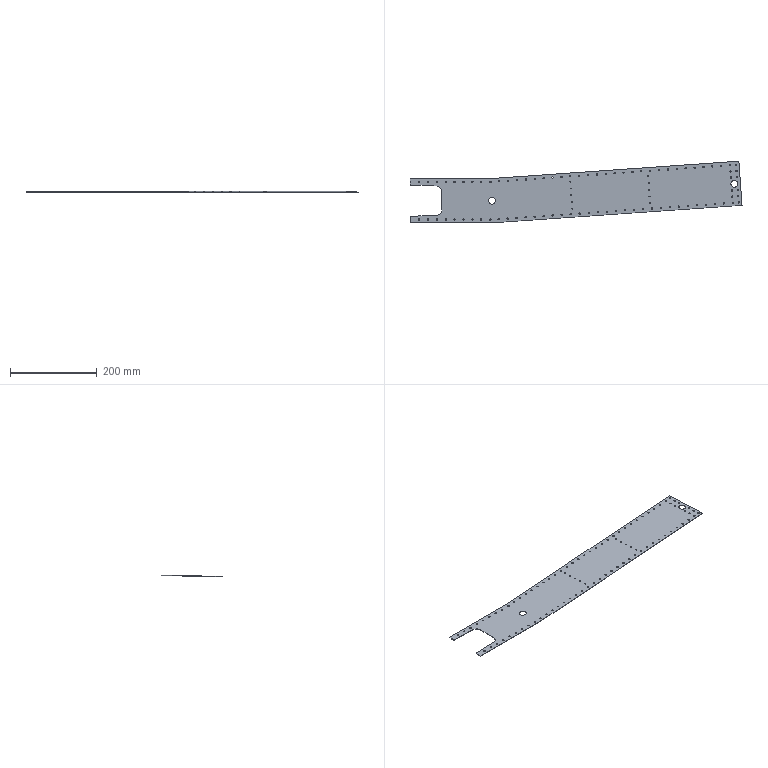Part | SolidWorks | features BaseBody 1 | 1 solid | 212 faces | box 764.943 x 141.945 x 3.277 mm | volume 57342 mm3 | cylinder 198 | plane 14 | commonest cylinder face diameters 3.2 x170 2.4 x20 15.9 x4 4 x2 26 x2